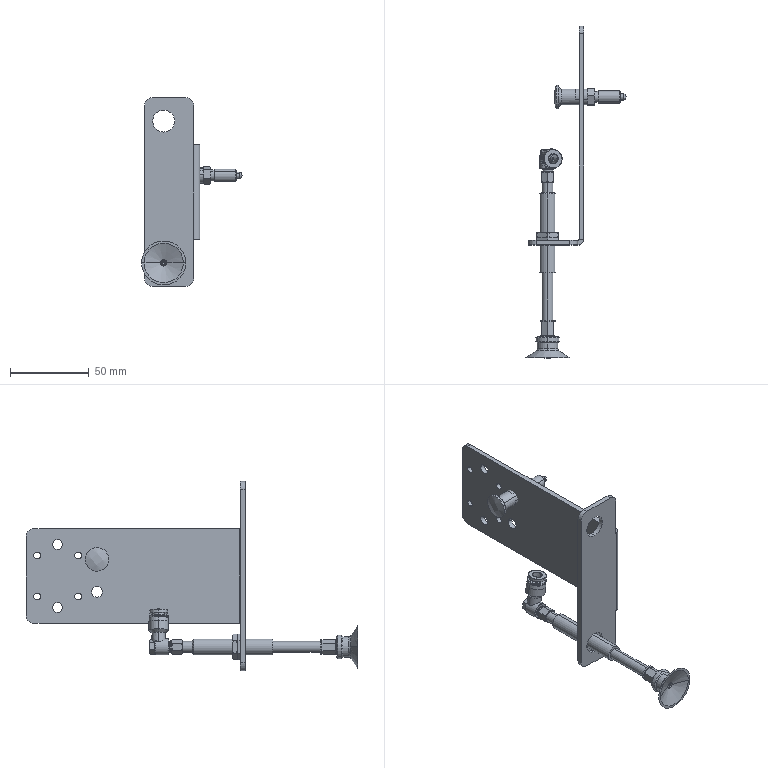Part | SolidWorks | features ReferencePattern 2, DerivedHolePattern 1 | 6 solids | 335 faces | box 63.895 x 210.5 x 120 mm | volume 48532 mm3 | cone 112 | plane 103 | cylinder 101 | spline 19 | commonest cylinder face diameters 7 x12 10 x12 4.2 x8 4 x6 5 x6 6 x6